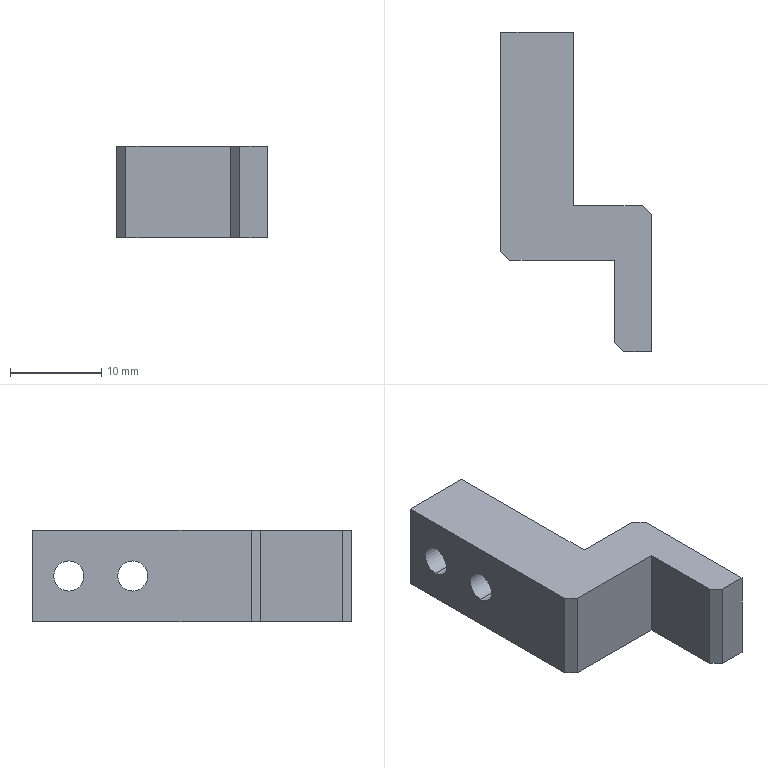Part | STEP file | PN_0058 Mount electronic clip electronic clip plate | 1 solid | 23 faces | box 16.5 x 35 x 10 mm | volume 2631 mm3 | plane 17 | cylinder 6 | commonest cylinder face diameters 3.3 x4 4 x2